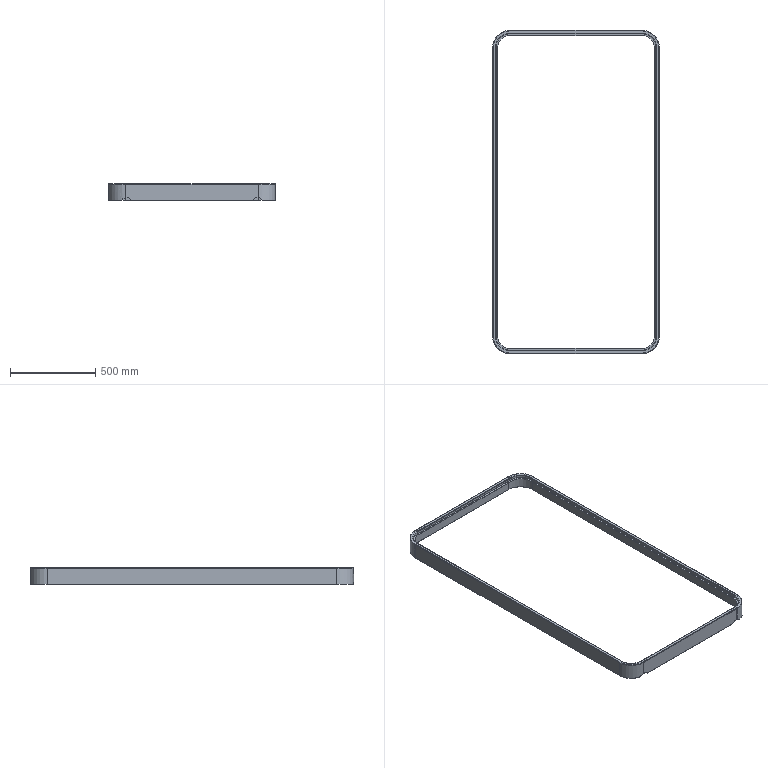Part | STEP file | Housing front face solid 001 | 1 solid | 64 faces | box 980 x 1900 x 96 mm | volume 1146713 mm3 | cylinder 30 | plane 26 | torus 8 | commonest cylinder face diameters 6 x8 140 x4 160 x4 163 x4 197 x4 200 x4